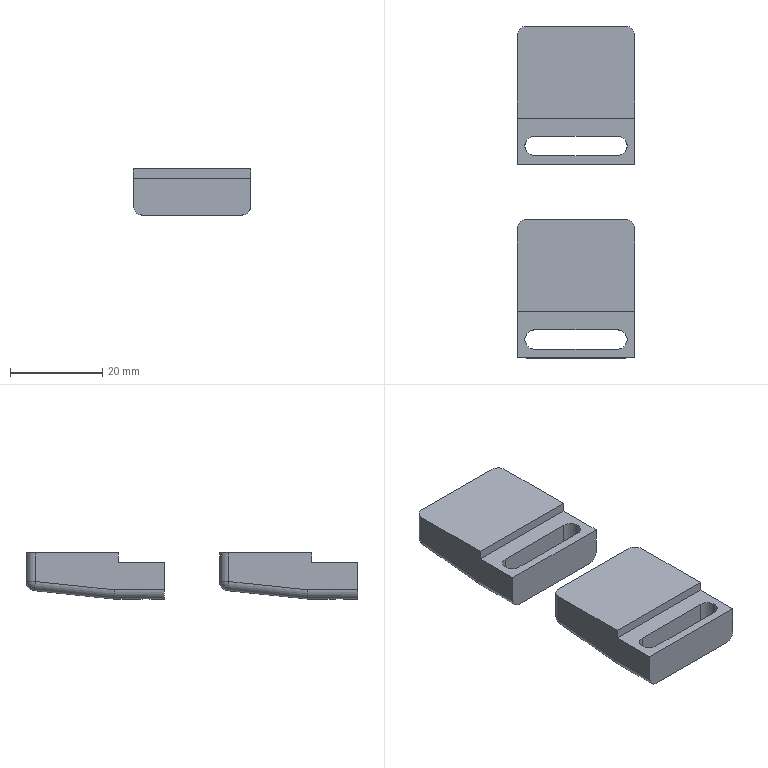NC program | NX | posted with a generic post | part box 25.5 x 72 x 10 mm
Lines 50360 to 51151 of 60534:
(FIXED_CONTOUR_COPY , TOOL : R2)
N100706 T18 M6
N100708 G54
N100710 G17 G0 G90 X23.999 Y-2.844 B0. C0. S9500 M3
N100712 G43 Z30. H18
N100714 Z2.8
N100716 G94 G1 Z-1.939 F1000.
N100718 X23.986 Y-2.857 Z-1.906 F2500.
N100720 X23.923 Y-2.92 Z-1.669
N100722 X23.857 Y-2.919 Z-1.674
N100724 X23.919 Y-2.857 Z-1.906
N100726 X24. Y-2.775 Z-2.113
N100728 Y-2.745 Z-2.188
N100730 Y-2.712 Z-2.252
N100732 Z-2.267
N100734 X23.915 Y-2.797 Z-2.061
N100736 X23.855 Y-2.857 Z-1.907
N100738 X23.794 Y-2.918 Z-1.678
N100740 X23.75 Y-2.917 Z-1.68
N100742 X23.811 Y-2.857 Z-1.907
N100744 X23.864 Y-2.803 Z-2.046
N100746 X23.974 Y-2.693 Z-2.311
N100748 X24. Y-2.668 Z-2.357
N100750 Z-2.339
N100752 Y-2.579 Z-2.512
N100754 X23.999 Z-2.515
N100756 X23.884 Y-2.693 Z-2.311
N100758 X23.837 Y-2.74 Z-2.199
N100760 X23.762 Y-2.815 Z-2.016
N100762 X23.724 Y-2.854 Z-1.915
N100764 X23.662 Y-2.916 Z-1.686
N100766 X23.596 Y-2.915 Z-1.69
N100768 X23.639 Y-2.872 Z-1.85
N100770 X23.664 Y-2.847 Z-1.932
N100772 X23.695 Y-2.816 Z-2.013
N100774 X23.795 Y-2.716 Z-2.259
N100776 X23.818 Y-2.693 Z-2.311
N100778 X23.977 Y-2.534 Z-2.594
N100780 X24. Y-2.511 Z-2.627
N100782 Z-2.618
N100784 Y-2.454 Z-2.701
N100786 Z-2.709
N100788 X23.923 Y-2.531 Z-2.599
N100790 X23.761 Y-2.693 Z-2.311
N100792 X23.738 Y-2.716 Z-2.259
N100794 X23.638 Y-2.816 Z-2.014
N100796 X23.613 Y-2.842 Z-1.947
N100798 X23.573 Y-2.881 Z-1.817
N100800 X23.54 Y-2.914 Z-1.694
N100802 X23.438 Y-2.913 Z-1.7
N100804 X23.453 Y-2.898 Z-1.756
N100806 X23.52 Y-2.832 Z-1.973
N100808 X23.635 Y-2.716 Z-2.26
N100810 X23.652 Y-2.699 Z-2.299
N100812 X23.825 Y-2.526 Z-2.609
N100814 X23.907 Y-2.444 Z-2.724
N100816 X24. Y-2.351 Z-2.85
N100818 Z-2.846
N100820 Y-2.288 Z-2.92
N100822 Z-2.927
N100824 X23.96 Y-2.328 Z-2.881
N100826 X23.844 Y-2.444 Z-2.724
N100828 X23.765 Y-2.523 Z-2.614
N100830 X23.642 Y-2.646 Z-2.393
N100832 X23.585 Y-2.703 Z-2.29
N100834 X23.463 Y-2.825 Z-1.989
N100836 X23.376 Y-2.912 Z-1.704
N100838 X23.273 Y-2.91 Z-1.71
N100840 X23.37 Y-2.814 Z-2.019
N100842 X23.474 Y-2.709 Z-2.276
N100844 X23.564 Y-2.619 Z-2.443
N100846 X23.661 Y-2.522 Z-2.615
N100848 X23.742 Y-2.441 Z-2.728
N100850 X23.855 Y-2.328 Z-2.881
N100852 X23.945 Y-2.238 Z-2.986
N100854 X23.998 Y-2.185 Z-3.042
N100856 Y-2.148 Z-3.08
N100858 X24. Y-2.089 Z-3.136
N100860 Z-3.142
N100862 X23.851 Y-2.238 Z-2.986
N100864 X23.761 Y-2.328 Z-2.881
N100866 X23.567 Y-2.522 Z-2.615
N100868 X23.47 Y-2.619 Z-2.443
N100870 X23.374 Y-2.715 Z-2.264
N100872 X23.276 Y-2.813 Z-2.021
N100874 X23.18 Y-2.909 Z-1.716
N100876 X23.078 Y-2.907 Z-1.723
N100878 X23.173 Y-2.812 Z-2.023
N100880 X23.269 Y-2.716 Z-2.262
N100882 X23.366 Y-2.619 Z-2.443
N100884 X23.463 Y-2.522 Z-2.615
N100886 X23.657 Y-2.328 Z-2.881
N100888 X23.748 Y-2.237 Z-2.987
N100890 X23.947 Y-2.038 Z-3.196
N100892 X24. Y-1.985 Z-3.239
N100894 X23.998 Y-1.883 Z-3.323
N100896 X23.843 Y-2.038 Z-3.196
N100898 X23.666 Y-2.216 Z-3.01
N100900 X23.553 Y-2.328 Z-2.881
N100902 X23.359 Y-2.522 Z-2.615
N100904 X23.232 Y-2.649 Z-2.388
N100906 X23.165 Y-2.716 Z-2.262
N100908 X23.07 Y-2.812 Z-2.025
N100910 X22.975 Y-2.906 Z-1.729
N100912 X22.872 Y-2.904 Z-1.736
N100914 X22.966 Y-2.811 Z-2.026
N100916 X23.06 Y-2.716 Z-2.263
N100918 X23.157 Y-2.619 Z-2.443
N100920 X23.254 Y-2.522 Z-2.615
N100922 X23.449 Y-2.328 Z-2.881
N100924 X23.583 Y-2.194 Z-3.032
N100926 X23.741 Y-2.036 Z-3.198
N100928 X23.978 Y-1.798 Z-3.392
N100930 X23.998 Y-1.778 Z-3.407
N100932 X24. Y-1.757 Z-3.422
N100934 Y-1.684 Z-3.468
N100936 Z-3.474
N100938 X23.885 Y-1.798 Z-3.392
N100940 X23.666 Y-2.017 Z-3.213
N100942 X23.611 Y-2.072 Z-3.16
N100944 X23.509 Y-2.175 Z-3.053
N100946 X23.355 Y-2.328 Z-2.88
N100948 X23.161 Y-2.522 Z-2.616
N100950 X23.064 Y-2.619 Z-2.443
N100952 X22.967 Y-2.716 Z-2.264
N100954 X22.873 Y-2.81 Z-2.028
N100956 X22.781 Y-2.903 Z-1.742
N100958 X22.697 Y-2.902 Z-1.747
N100960 X22.789 Y-2.81 Z-2.03
N100962 X22.883 Y-2.716 Z-2.264
N100964 X22.98 Y-2.619 Z-2.443
N100966 X23.077 Y-2.522 Z-2.616
N100968 X23.271 Y-2.328 Z-2.881
N100970 X23.442 Y-2.157 Z-3.071
N100972 X23.5 Y-2.099 Z-3.132
N100974 X23.598 Y-2. Z-3.227
N100976 X23.8 Y-1.798 Z-3.392
N100978 X23.878 Y-1.721 Z-3.45
N100980 X24. Y-1.599 Z-3.527
N100982 Z-3.52
N100984 Y-1.514 Z-3.573
N100986 Z-3.58
N100988 X23.772 Y-1.742 Z-3.437
N100990 X23.53 Y-1.984 Z-3.241
N100992 X23.375 Y-2.139 Z-3.09
N100994 X23.186 Y-2.328 Z-2.881
N100996 X22.992 Y-2.522 Z-2.616
N100998 X22.875 Y-2.639 Z-2.406
N101000 X22.798 Y-2.716 Z-2.264
N101002 X22.705 Y-2.809 Z-2.031
N101004 X22.614 Y-2.9 Z-1.752
N101006 X22.511 Y-2.899 Z-1.759
N101008 X22.601 Y-2.808 Z-2.033
N101010 X22.694 Y-2.716 Z-2.265
N101012 X22.791 Y-2.619 Z-2.443
N101014 X22.888 Y-2.522 Z-2.616
N101016 X23.082 Y-2.328 Z-2.881
N101018 X23.276 Y-2.134 Z-3.095
N101020 X23.447 Y-1.963 Z-3.258
N101022 X23.664 Y-1.746 Z-3.435
N101024 X23.971 Y-1.439 Z-3.627
N101026 X24. Y-1.41 Z-3.641
N101028 Z-3.638
N101030 X23.998 Y-1.382 Z-3.655
N101032 X24. Y-1.334 Z-3.676
N101034 Y-1.306 Z-3.688
N101036 Z-3.691
N101038 X23.867 Y-1.439 Z-3.627
N101040 X23.56 Y-1.746 Z-3.435
N101042 X23.354 Y-1.951 Z-3.266
N101044 X23.171 Y-2.134 Z-3.095
N101046 X22.977 Y-2.328 Z-2.881
N101048 X22.783 Y-2.522 Z-2.616
N101050 X22.686 Y-2.619 Z-2.443
N101052 X22.589 Y-2.716 Z-2.265
N101054 X22.498 Y-2.808 Z-2.035
N101056 X22.408 Y-2.897 Z-1.765
N101058 X22.319 Y-2.896 Z-1.771
N101060 X22.408 Y-2.807 Z-2.036
N101062 X22.499 Y-2.716 Z-2.265
N101064 X22.596 Y-2.619 Z-2.443
N101066 X22.693 Y-2.522 Z-2.616
N101068 X22.887 Y-2.328 Z-2.881
N101070 X23.081 Y-2.134 Z-3.095
N101072 X23.275 Y-1.94 Z-3.276
N101074 X23.469 Y-1.746 Z-3.435
N101076 X23.776 Y-1.439 Z-3.627
N101078 X24. Y-1.215 Z-3.733
N101080 Z-3.726
N101082 Y-1.124 Z-3.765
N101084 Z-3.774
N101086 X23.696 Y-1.428 Z-3.633
N101088 X23.658 Y-1.465 Z-3.611
N101090 X23.378 Y-1.746 Z-3.435
N101092 X23.184 Y-1.94 Z-3.276
N101094 X22.99 Y-2.134 Z-3.095
N101096 X22.796 Y-2.328 Z-2.881
N101098 X22.602 Y-2.522 Z-2.616
N101100 X22.505 Y-2.619 Z-2.443
N101102 X22.408 Y-2.716 Z-2.266
N101104 X22.318 Y-2.806 Z-2.038
N101106 X22.229 Y-2.895 Z-1.776
N101108 X22.127 Y-2.893 Z-1.783
N101110 X22.214 Y-2.805 Z-2.04
N101112 X22.304 Y-2.716 Z-2.266
N101114 X22.432 Y-2.588 Z-2.499
N101116 X22.498 Y-2.522 Z-2.616
N101118 X22.692 Y-2.328 Z-2.881
N101120 X22.886 Y-2.134 Z-3.095
N101122 X23.08 Y-1.94 Z-3.276
N101124 X23.274 Y-1.746 Z-3.435
N101126 X23.513 Y-1.507 Z-3.585
N101128 X23.61 Y-1.41 Z-3.641
N101130 X23.856 Y-1.164 Z-3.757
N101132 X23.946 Y-1.074 Z-3.796
N101134 X24. Y-1.02 Z-3.813
N101136 Z-3.81
N101138 X23.998 Y-0.987 Z-3.824
N101140 X24. Y-0.961 Z-3.832
N101142 Y-0.916 Z-3.843
N101144 Z-3.846
N101146 X23.842 Y-1.074 Z-3.796
N101148 X23.751 Y-1.164 Z-3.756
N101150 X23.524 Y-1.392 Z-3.65
N101152 X23.368 Y-1.548 Z-3.559
N101154 X23.17 Y-1.746 Z-3.435
N101156 X22.976 Y-1.94 Z-3.276
N101158 X22.782 Y-2.134 Z-3.095
N101160 X22.588 Y-2.328 Z-2.881
N101162 X22.394 Y-2.522 Z-2.616
N101164 X22.2 Y-2.716 Z-2.266
N101166 X22.111 Y-2.805 Z-2.042
N101168 X22.024 Y-2.892 Z-1.789
N101170 X21.93 Y-2.89 Z-1.795
N101172 X22.017 Y-2.804 Z-2.044
N101174 X22.104 Y-2.716 Z-2.266
N101176 X22.299 Y-2.522 Z-2.617
N101178 X22.493 Y-2.328 Z-2.881
N101180 X22.687 Y-2.134 Z-3.095
N101182 X22.881 Y-1.94 Z-3.276
N101184 X23.075 Y-1.746 Z-3.435
N101186 X23.269 Y-1.552 Z-3.556
N101188 X23.445 Y-1.376 Z-3.658
N101190 X23.657 Y-1.164 Z-3.757
N101192 X23.688 Y-1.133 Z-3.768
N101194 X23.748 Y-1.073 Z-3.796
N101196 X24. Y-0.821 Z-3.877
N101198 Z-3.869
N101200 Y-0.725 Z-3.895
N101202 Z-3.904
N101204 X23.949 Y-0.776 Z-3.892
N101206 X23.672 Y-1.053 Z-3.803
N101208 X23.623 Y-1.101 Z-3.78
N101210 X23.561 Y-1.164 Z-3.757
N101212 X23.354 Y-1.37 Z-3.659
N101214 X23.173 Y-1.552 Z-3.556
N101216 X22.979 Y-1.746 Z-3.435
N101218 X22.784 Y-1.94 Z-3.276
N101220 X22.59 Y-2.134 Z-3.095
N101222 X22.396 Y-2.328 Z-2.881
N101224 X22.202 Y-2.522 Z-2.617
N101226 X22.008 Y-2.716 Z-2.266
N101228 X21.921 Y-2.803 Z-2.045
N101230 X21.835 Y-2.889 Z-1.801
N101232 X21.733 Y-2.888 Z-1.808
N101234 X21.818 Y-2.802 Z-2.047
N101236 X21.905 Y-2.716 Z-2.266
N101238 X22.099 Y-2.522 Z-2.617
N101240 X22.293 Y-2.328 Z-2.881
N101242 X22.487 Y-2.134 Z-3.095
N101244 X22.681 Y-1.94 Z-3.276
N101246 X22.875 Y-1.746 Z-3.435
N101248 X23.069 Y-1.552 Z-3.556
N101250 X23.263 Y-1.358 Z-3.666
N101252 X23.457 Y-1.164 Z-3.757
N101254 X23.554 Y-1.067 Z-3.793
N101256 X23.59 Y-1.031 Z-3.809
N101258 X23.845 Y-0.776 Z-3.892
N101260 X23.935 Y-0.686 Z-3.914
N101262 X24. Y-0.621 Z-3.926
N101264 Z-3.923
N101266 X23.998 Y-0.592 Z-3.931
N101268 X24. Y-0.557 Z-3.938
N101270 Y-0.518 Z-3.943
N101272 Z-3.945
N101274 X23.832 Y-0.686 Z-3.914
N101276 X23.742 Y-0.776 Z-3.892
N101278 X23.507 Y-1.01 Z-3.816
N101280 X23.484 Y-1.033 Z-3.806
N101282 X23.353 Y-1.165 Z-3.756
N101284 X23.159 Y-1.358 Z-3.666
N101286 X22.965 Y-1.552 Z-3.556
N101288 X22.771 Y-1.746 Z-3.435
N101290 X22.577 Y-1.94 Z-3.276
N101292 X22.383 Y-2.134 Z-3.095
N101294 X22.189 Y-2.328 Z-2.881
N101296 X21.995 Y-2.522 Z-2.617
N101298 X21.801 Y-2.716 Z-2.266
N101300 X21.716 Y-2.802 Z-2.049
N101302 X21.631 Y-2.886 Z-1.814
N101304 X21.534 Y-2.885 Z-1.82
N101306 X21.618 Y-2.801 Z-2.051
N101308 X21.703 Y-2.716 Z-2.266
N101310 X21.897 Y-2.522 Z-2.618
N101312 X22.091 Y-2.328 Z-2.881
N101314 X22.285 Y-2.134 Z-3.095
N101316 X22.479 Y-1.94 Z-3.276
N101318 X22.673 Y-1.746 Z-3.435
N101320 X22.867 Y-1.552 Z-3.556
N101322 X23.061 Y-1.358 Z-3.666
N101324 X23.255 Y-1.164 Z-3.757
N101326 X23.43 Y-0.989 Z-3.823
N101328 X23.643 Y-0.776 Z-3.892
N101330 X23.737 Y-0.682 Z-3.914
N101332 X24. Y-0.419 Z-3.964
N101334 Z-3.958
N101336 Y-0.32 Z-3.973
N101338 Z-3.978
N101340 X23.933 Y-0.388 Z-3.97
N101342 X23.659 Y-0.661 Z-3.918
N101344 X23.544 Y-0.776 Z-3.892
N101346 X23.35 Y-0.97 Z-3.829
N101348 X23.156 Y-1.164 Z-3.757
N101350 X22.962 Y-1.358 Z-3.666
N101352 X22.768 Y-1.552 Z-3.556
N101354 X22.574 Y-1.746 Z-3.435
N101356 X22.38 Y-1.94 Z-3.276
N101358 X22.186 Y-2.134 Z-3.095
N101360 X21.992 Y-2.328 Z-2.881
N101362 X21.798 Y-2.522 Z-2.618
N101364 X21.604 Y-2.716 Z-2.266
N101366 X21.52 Y-2.8 Z-2.053
N101368 X21.437 Y-2.883 Z-1.827
N101370 X21.335 Y-2.882 Z-1.833
N101372 X21.417 Y-2.799 Z-2.055
N101374 X21.5 Y-2.716 Z-2.266
N101376 X21.694 Y-2.522 Z-2.618
N101378 X21.888 Y-2.328 Z-2.881
N101380 X22.082 Y-2.134 Z-3.095
N101382 X22.277 Y-1.94 Z-3.276
N101384 X22.471 Y-1.746 Z-3.435
N101386 X22.665 Y-1.552 Z-3.556
N101388 X22.859 Y-1.358 Z-3.666
N101390 X23.053 Y-1.164 Z-3.757
N101392 X23.247 Y-0.97 Z-3.829
N101394 X23.441 Y-0.776 Z-3.892
N101396 X23.577 Y-0.64 Z-3.922
N101398 X23.829 Y-0.388 Z-3.97
N101400 X24. Y-0.217 Z-3.99
N101402 Y-0.168 Z-3.992
N101404 Y-0.113
N101406 Z-3.995
N101408 X23.877 Y-0.235 Z-3.989
N101410 X23.725 Y-0.388 Z-3.97
N101412 X23.494 Y-0.618 Z-3.926
N101414 X23.337 Y-0.776 Z-3.892
N101416 X23.143 Y-0.97 Z-3.829
N101418 X22.949 Y-1.164 Z-3.757
N101420 X22.755 Y-1.358 Z-3.666
N101422 X22.56 Y-1.552 Z-3.556
N101424 X22.367 Y-1.746 Z-3.435
N101426 X22.173 Y-1.94 Z-3.276
N101428 X21.978 Y-2.134 Z-3.095
N101430 X21.784 Y-2.328 Z-2.881
N101432 X21.59 Y-2.522 Z-2.618
N101434 X21.396 Y-2.716 Z-2.266
N101436 X21.314 Y-2.799 Z-2.058
N101438 X21.233 Y-2.88 Z-1.839
N101440 X21.135 Y-2.878 Z-1.846
N101442 X21.215 Y-2.798 Z-2.061
N101444 X21.296 Y-2.716 Z-2.266
N101446 X21.49 Y-2.522 Z-2.618
N101448 X21.684 Y-2.328 Z-2.881
N101450 X21.879 Y-2.134 Z-3.095
N101452 X22.073 Y-1.94 Z-3.276
N101454 X22.267 Y-1.746 Z-3.435
N101456 X22.461 Y-1.552 Z-3.556
N101458 X22.655 Y-1.358 Z-3.666
N101460 X22.849 Y-1.164 Z-3.757
N101462 X23.043 Y-0.97 Z-3.829
N101464 X23.237 Y-0.776 Z-3.892
N101466 X23.415 Y-0.598 Z-3.93
N101468 X23.625 Y-0.388 Z-3.97
N101470 X23.809 Y-0.203 Z-3.992
N101472 X24. Y-0.013 Z-3.999
N101474 Z-3.992
N101476 Y0.087
N101478 Z-3.996
N101480 X23.913 Y0.001 Z-3.999
N101482 X23.719 Y-0.193 Z-3.993
N101484 X23.525 Y-0.388 Z-3.97
N101486 X23.331 Y-0.582 Z-3.933
N101488 X23.137 Y-0.776 Z-3.892
N101490 X22.943 Y-0.97 Z-3.829
N101492 X22.749 Y-1.164 Z-3.757
N101494 X22.555 Y-1.358 Z-3.666
N101496 X22.361 Y-1.552 Z-3.556
N101498 X22.167 Y-1.746 Z-3.435
N101500 X21.973 Y-1.94 Z-3.276
N101502 X21.779 Y-2.134 Z-3.095
N101504 X21.584 Y-2.328 Z-2.881
N101506 X21.39 Y-2.522 Z-2.619
N101508 X21.196 Y-2.716 Z-2.266
N101510 X21.116 Y-2.797 Z-2.064
N101512 X21.037 Y-2.876 Z-1.852
N101514 X20.934 Y-2.874 Z-1.858
N101516 X21.022 Y-2.785 Z-2.094
N101518 X21.091 Y-2.716 Z-2.266
N101520 X21.285 Y-2.522 Z-2.619
N101522 X21.479 Y-2.328 Z-2.881
N101524 X21.673 Y-2.134 Z-3.095
N101526 X21.867 Y-1.94 Z-3.276
N101528 X22.061 Y-1.746 Z-3.435
N101530 X22.256 Y-1.552 Z-3.556
N101532 X22.45 Y-1.358 Z-3.666
N101534 X22.644 Y-1.164 Z-3.757
N101536 X22.838 Y-0.97 Z-3.829
N101538 X23.032 Y-0.776 Z-3.892
N101540 X23.226 Y-0.582 Z-3.933
N101542 X23.42 Y-0.388 Z-3.97
N101544 X23.614 Y-0.193 Z-3.993
N101546 X23.808 Y0.001 Z-3.999
N101548 X23.998 Y0.191 Z-3.991
N101550 X24. Y0.218 Z-3.989
N101552 Y0.298 Z-3.977
N101554 Z-3.981
N101556 X23.926 Y0.224 Z-3.99
N101558 X23.796 Y0.094 Z-3.996
N101560 X23.702 Y0.001 Z-3.999
N101562 X23.494 Y-0.208 Z-3.991
N101564 X23.314 Y-0.388 Z-3.97
N101566 X23.12 Y-0.582 Z-3.933
N101568 X22.926 Y-0.776 Z-3.892
N101570 X22.732 Y-0.97 Z-3.829
N101572 X22.538 Y-1.164 Z-3.757
N101574 X22.344 Y-1.358 Z-3.666
N101576 X22.15 Y-1.552 Z-3.556
N101578 X21.956 Y-1.746 Z-3.435
N101580 X21.762 Y-1.94 Z-3.276
N101582 X21.568 Y-2.134 Z-3.095
N101584 X21.374 Y-2.328 Z-2.881
N101586 X21.18 Y-2.522 Z-2.619
N101588 X20.986 Y-2.716 Z-2.266
N101590 X20.892 Y-2.809 Z-2.031
N101592 X20.83 Y-2.872 Z-1.865
N101594 X20.727 Y-2.87 Z-1.871
N101596 X20.803 Y-2.794 Z-2.074
N101598 X20.88 Y-2.716 Z-2.266
N101600 X21.074 Y-2.522 Z-2.619
N101602 X21.268 Y-2.328 Z-2.881
N101604 X21.462 Y-2.134 Z-3.095
N101606 X21.656 Y-1.94 Z-3.276
N101608 X21.85 Y-1.746 Z-3.435
N101610 X22.044 Y-1.552 Z-3.556
N101612 X22.238 Y-1.358 Z-3.666
N101614 X22.433 Y-1.164 Z-3.757
N101616 X22.627 Y-0.97 Z-3.829
N101618 X22.821 Y-0.776 Z-3.892
N101620 X23.015 Y-0.582 Z-3.933
N101622 X23.209 Y-0.388 Z-3.97
N101624 X23.403 Y-0.193 Z-3.993
N101626 X23.597 Y0.001 Z-3.999
N101628 X23.799 Y0.203 Z-3.992
N101630 X24. Y0.403 Z-3.967
N101632 Z-3.96
N101634 Y0.509 Z-3.944
N101636 Z-3.947
N101638 X23.879 Y0.389 Z-3.97
N101640 X23.685 Y0.195 Z-3.992
N101642 X23.491 Y0.001 Z-3.999
N101644 X23.297 Y-0.193 Z-3.993
N101646 X23.103 Y-0.388 Z-3.97
N101648 X22.909 Y-0.582 Z-3.933
N101650 X22.715 Y-0.776 Z-3.892
N101652 X22.521 Y-0.97 Z-3.829
N101654 X22.327 Y-1.164 Z-3.757
N101656 X22.133 Y-1.358 Z-3.666
N101658 X21.939 Y-1.552 Z-3.556
N101660 X21.745 Y-1.746 Z-3.435
N101662 X21.551 Y-1.94 Z-3.276
N101664 X21.357 Y-2.134 Z-3.095
N101666 X21.163 Y-2.328 Z-2.881
N101668 X20.969 Y-2.522 Z-2.619
N101670 X20.774 Y-2.716 Z-2.266
N101672 X20.698 Y-2.793 Z-2.078
N101674 X20.623 Y-2.867 Z-1.878
N101676 X20.52 Y-2.865 Z-1.884
N101678 X20.594 Y-2.791 Z-2.081
N101680 X20.669 Y-2.716 Z-2.266
N101682 X20.863 Y-2.522 Z-2.619
N101684 X21.057 Y-2.328 Z-2.881
N101686 X21.251 Y-2.134 Z-3.095
N101688 X21.445 Y-1.94 Z-3.276
N101690 X21.639 Y-1.746 Z-3.435
N101692 X21.833 Y-1.552 Z-3.556
N101694 X22.027 Y-1.358 Z-3.666
N101696 X22.221 Y-1.164 Z-3.757
N101698 X22.415 Y-0.97 Z-3.829
N101700 X22.609 Y-0.776 Z-3.892
N101702 X22.803 Y-0.582 Z-3.933
N101704 X22.997 Y-0.388 Z-3.97
N101706 X23.192 Y-0.193 Z-3.993
N101708 X23.386 Y0.001 Z-3.999
N101710 X23.58 Y0.195 Z-3.992
N101712 X23.774 Y0.389 Z-3.97
N101714 X24. Y0.615 Z-3.927
N101716 Z-3.925
N101718 Y0.715 Z-3.898
N101720 Z-3.907
N101722 X23.972 Y0.687 Z-3.913
N101724 X23.674 Y0.389 Z-3.97
N101726 X23.48 Y0.195 Z-3.992
N101728 X23.286 Y0.001 Z-3.999
N101730 X23.092 Y-0.193 Z-3.993
N101732 X22.897 Y-0.388 Z-3.97
N101734 X22.703 Y-0.582 Z-3.933
N101736 X22.509 Y-0.776 Z-3.892
N101738 X22.315 Y-0.97 Z-3.829
N101740 X22.121 Y-1.164 Z-3.757
N101742 X21.927 Y-1.358 Z-3.666
N101744 X21.733 Y-1.552 Z-3.556
N101746 X21.539 Y-1.746 Z-3.435
N101748 X21.345 Y-1.94 Z-3.276
N101750 X21.151 Y-2.134 Z-3.095
N101752 X20.957 Y-2.328 Z-2.881
N101754 X20.763 Y-2.522 Z-2.619
N101756 X20.569 Y-2.716 Z-2.266
N101758 X20.494 Y-2.79 Z-2.084
N101760 X20.422 Y-2.863 Z-1.891
N101762 X20.323 Y-2.862 Z-1.897
N101764 X20.395 Y-2.79 Z-2.088
N101766 X20.469 Y-2.716 Z-2.267
N101768 X20.663 Y-2.522 Z-2.619
N101770 X20.857 Y-2.328 Z-2.881
N101772 X21.051 Y-2.134 Z-3.095
N101774 X21.245 Y-1.94 Z-3.276
N101776 X21.439 Y-1.746 Z-3.435
N101778 X21.633 Y-1.552 Z-3.556
N101780 X21.827 Y-1.358 Z-3.666
N101782 X22.021 Y-1.164 Z-3.757
N101784 X22.215 Y-0.97 Z-3.829
N101786 X22.409 Y-0.776 Z-3.892
N101788 X22.603 Y-0.582 Z-3.933
N101790 X22.797 Y-0.388 Z-3.97
N101792 X22.992 Y-0.193 Z-3.993
N101794 X23.186 Y0.001 Z-3.999
N101796 X23.38 Y0.195 Z-3.992
N101798 X23.574 Y0.389 Z-3.97
N101800 X23.872 Y0.687 Z-3.913
N101802 X23.962 Y0.777 Z-3.891
N101804 X24. Y0.815 Z-3.879
N101806 Z-3.871
N101808 Y0.915 Z-3.843
N101810 Z-3.847
N101812 X23.862 Y0.777 Z-3.891
N101814 X23.751 Y0.666 Z-3.917
N101816 X23.474 Y0.389 Z-3.97
N101818 X23.28 Y0.195 Z-3.992
N101820 X23.086 Y0.001 Z-3.999
N101822 X22.892 Y-0.193 Z-3.993
N101824 X22.697 Y-0.388 Z-3.97
N101826 X22.503 Y-0.582 Z-3.933
N101828 X22.309 Y-0.776 Z-3.892
N101830 X22.115 Y-0.97 Z-3.829
N101832 X21.921 Y-1.164 Z-3.757
N101834 X21.727 Y-1.358 Z-3.666
N101836 X21.533 Y-1.552 Z-3.556
N101838 X21.339 Y-1.746 Z-3.435
N101840 X21.145 Y-1.94 Z-3.276
N101842 X20.951 Y-2.134 Z-3.095
N101844 X20.757 Y-2.328 Z-2.881
N101846 X20.563 Y-2.522 Z-2.619
N101848 X20.369 Y-2.716 Z-2.267
N101850 X20.296 Y-2.789 Z-2.091
N101852 X20.226 Y-2.859 Z-1.903
N101854 X20.122 Y-2.858 Z-1.909
N101856 X20.192 Y-2.787 Z-2.094
N101858 X20.263 Y-2.716 Z-2.267
N101860 X20.457 Y-2.522 Z-2.619
N101862 X20.651 Y-2.328 Z-2.881
N101864 X20.845 Y-2.134 Z-3.095
N101866 X21.039 Y-1.94 Z-3.276
N101868 X21.233 Y-1.746 Z-3.435
N101870 X21.427 Y-1.552 Z-3.556
N101872 X21.621 Y-1.358 Z-3.666
N101874 X21.815 Y-1.164 Z-3.757
N101876 X22.009 Y-0.97 Z-3.829
N101878 X22.203 Y-0.776 Z-3.892
N101880 X22.398 Y-0.582 Z-3.933
N101882 X22.592 Y-0.388 Z-3.97
N101884 X22.786 Y-0.193 Z-3.993
N101886 X22.98 Y0.001 Z-3.999
N101888 X23.174 Y0.195 Z-3.992
N101890 X23.368 Y0.389 Z-3.97
N101892 X23.682 Y0.703 Z-3.91
N101894 X23.755 Y0.776 Z-3.892
N101896 X24. Y1.021 Z-3.813
N101898 Z-3.809
N101900 Y1.12 Z-3.767
N101902 Z-3.776
N101904 X23.954 Y1.075 Z-3.795
N101906 X23.656 Y0.777 Z-3.891
N101908 X23.6 Y0.721 Z-3.905
N101910 X23.268 Y0.389 Z-3.97
N101912 X23.074 Y0.195 Z-3.992
N101914 X22.88 Y0.001 Z-3.999
N101916 X22.686 Y-0.193 Z-3.993
N101918 X22.492 Y-0.388 Z-3.97
N101920 X22.298 Y-0.582 Z-3.933
N101922 X22.104 Y-0.776 Z-3.892
N101924 X21.909 Y-0.97 Z-3.829
N101926 X21.715 Y-1.164 Z-3.757
N101928 X21.521 Y-1.358 Z-3.666
N101930 X21.327 Y-1.552 Z-3.556
N101932 X21.133 Y-1.746 Z-3.435
N101934 X20.939 Y-1.94 Z-3.276
N101936 X20.745 Y-2.134 Z-3.095
N101938 X20.551 Y-2.328 Z-2.881
N101940 X20.357 Y-2.522 Z-2.619
N101942 X20.163 Y-2.716 Z-2.267
N101944 X20.093 Y-2.786 Z-2.098
N101946 X20.024 Y-2.856 Z-1.916
N101948 X19.926 Y-2.854 Z-1.922
N101950 X19.994 Y-2.785 Z-2.101
N101952 X20.063 Y-2.716 Z-2.267
N101954 X20.257 Y-2.522 Z-2.619
N101956 X20.451 Y-2.328 Z-2.881
N101958 X20.645 Y-2.134 Z-3.095
N101960 X20.839 Y-1.94 Z-3.276
N101962 X21.033 Y-1.746 Z-3.435
N101964 X21.227 Y-1.552 Z-3.556
N101966 X21.421 Y-1.358 Z-3.666
N101968 X21.615 Y-1.164 Z-3.757
N101970 X21.81 Y-0.97 Z-3.829
N101972 X22.004 Y-0.776 Z-3.892
N101974 X22.198 Y-0.582 Z-3.933
N101976 X22.392 Y-0.388 Z-3.97
N101978 X22.586 Y-0.193 Z-3.993
N101980 X22.78 Y0.001 Z-3.999
N101982 X22.974 Y0.195 Z-3.992
N101984 X23.168 Y0.389 Z-3.97
N101986 X23.359 Y0.58 Z-3.934
N101988 X23.556 Y0.777 Z-3.891
N101990 X23.854 Y1.075 Z-3.795
N101992 X24. Y1.22 Z-3.73
N101994 Z-3.724
N101996 Y1.32 Z-3.682
N101998 Z-3.683
N102000 X23.845 Y1.165 Z-3.756
N102002 X23.754 Y1.074 Z-3.796
N102004 X23.456 Y0.777 Z-3.891
N102006 X23.262 Y0.583 Z-3.933
N102008 X23.068 Y0.389 Z-3.97
N102010 X22.874 Y0.195 Z-3.992
N102012 X22.68 Y0.001 Z-3.999
N102014 X22.486 Y-0.193 Z-3.993
N102016 X22.292 Y-0.388 Z-3.97
N102018 X22.098 Y-0.582 Z-3.933
N102020 X21.904 Y-0.776 Z-3.892
N102022 X21.71 Y-0.97 Z-3.829
N102024 X21.516 Y-1.164 Z-3.757
N102026 X21.322 Y-1.358 Z-3.666
N102028 X21.128 Y-1.552 Z-3.556
N102030 X20.934 Y-1.746 Z-3.435
N102032 X20.74 Y-1.94 Z-3.276
N102034 X20.546 Y-2.134 Z-3.095
N102036 X20.351 Y-2.328 Z-2.881
N102038 X20.157 Y-2.522 Z-2.619
N102040 X19.963 Y-2.716 Z-2.267
N102042 X19.895 Y-2.784 Z-2.104
N102044 X19.828 Y-2.852 Z-1.928
N102046 X19.731 Y-2.85 Z-1.934
N102048 X19.797 Y-2.784 Z-2.107
N102050 X19.864 Y-2.716 Z-2.267
N102052 X20.058 Y-2.522 Z-2.619
N102054 X20.252 Y-2.328 Z-2.881
N102056 X20.446 Y-2.134 Z-3.095
N102058 X20.641 Y-1.94 Z-3.276
N102060 X20.835 Y-1.746 Z-3.435
N102062 X21.029 Y-1.552 Z-3.556
N102064 X21.223 Y-1.358 Z-3.666
N102066 X21.417 Y-1.164 Z-3.757
N102068 X21.611 Y-0.97 Z-3.829
N102070 X21.805 Y-0.776 Z-3.892
N102072 X21.999 Y-0.582 Z-3.933
N102074 X22.193 Y-0.388 Z-3.97
N102076 X22.387 Y-0.193 Z-3.993
N102078 X22.581 Y0.001 Z-3.999
N102080 X22.775 Y0.195 Z-3.992
N102082 X22.969 Y0.389 Z-3.97
N102084 X23.163 Y0.583 Z-3.933
N102086 X23.357 Y0.776 Z-3.891
N102088 X23.621 Y1.041 Z-3.806
N102090 X23.673 Y1.093 Z-3.788
N102092 X23.857 Y1.276 Z-3.704
N102094 X24. Y1.419 Z-3.637
N102096 Z-3.632
N102098 Y1.525 Z-3.566
N102100 Z-3.573
N102102 X23.914 Y1.439 Z-3.627
N102104 X23.64 Y1.165 Z-3.756
N102106 X23.587 Y1.112 Z-3.779
N102108 X23.478 Y1.003 Z-3.818
N102110 X23.252 Y0.777 Z-3.891
N102112 X23.058 Y0.583 Z-3.933
N102114 X22.863 Y0.389 Z-3.97
N102116 X22.669 Y0.195 Z-3.992
N102118 X22.475 Y0.001 Z-3.999
N102120 X22.281 Y-0.193 Z-3.993
N102122 X22.087 Y-0.388 Z-3.97
N102124 X21.893 Y-0.582 Z-3.933
N102126 X21.699 Y-0.776 Z-3.892
N102128 X21.505 Y-0.97 Z-3.829
N102130 X21.311 Y-1.164 Z-3.757
N102132 X21.117 Y-1.358 Z-3.666
N102134 X20.923 Y-1.552 Z-3.556
N102136 X20.729 Y-1.746 Z-3.435
N102138 X20.535 Y-1.94 Z-3.276
N102140 X20.341 Y-2.134 Z-3.095
N102142 X20.147 Y-2.328 Z-2.881
N102144 X19.953 Y-2.522 Z-2.619
N102146 X19.759 Y-2.716 Z-2.267
N102148 X19.676 Y-2.799 Z-2.068
N102150 X19.627 Y-2.847 Z-1.941
N102152 X19.524 Y-2.845 Z-1.947
N102154 X19.614 Y-2.755 Z-2.175
N102156 X19.653 Y-2.716 Z-2.267
N102158 X19.847 Y-2.522 Z-2.619
N102160 X20.041 Y-2.328 Z-2.881
N102162 X20.235 Y-2.134 Z-3.095
N102164 X20.429 Y-1.94 Z-3.276
N102166 X20.623 Y-1.746 Z-3.435
N102168 X20.817 Y-1.552 Z-3.556
N102170 X21.011 Y-1.358 Z-3.666
N102172 X21.205 Y-1.164 Z-3.757
N102174 X21.399 Y-0.97 Z-3.829
N102176 X21.593 Y-0.776 Z-3.892
N102178 X21.787 Y-0.582 Z-3.933
N102180 X21.981 Y-0.388 Z-3.97
N102182 X22.175 Y-0.193 Z-3.993
N102184 X22.369 Y0.001 Z-3.999
N102186 X22.562 Y0.194 Z-3.993
N102188 X22.758 Y0.389 Z-3.97
N102190 X22.952 Y0.583 Z-3.933
N102192 X23.146 Y0.777 Z-3.891
N102194 X23.354 Y0.985 Z-3.823
N102196 X23.501 Y1.132 Z-3.771
N102198 X23.808 Y1.439 Z-3.627
N102200 X24. Y1.631 Z-3.507
N102202 Z-3.5
N102204 Y1.737 Z-3.435
N102206 Z-3.437
N102208 X23.961 Y1.698 Z-3.465
N102210 X23.751 Y1.488 Z-3.596
N102212 X23.69 Y1.427 Z-3.633
N102214 X23.414 Y1.151 Z-3.762
N102216 X23.234 Y0.971 Z-3.829
N102218 X23.04 Y0.777 Z-3.891
N102220 X22.846 Y0.583 Z-3.933
N102222 X22.652 Y0.389 Z-3.97
N102224 X22.458 Y0.195 Z-3.992
N102226 X22.264 Y0.001 Z-3.999
N102228 X22.07 Y-0.193 Z-3.993
N102230 X21.876 Y-0.388 Z-3.97
N102232 X21.682 Y-0.582 Z-3.933
N102234 X21.487 Y-0.776 Z-3.892
N102236 X21.293 Y-0.97 Z-3.829
N102238 X21.099 Y-1.164 Z-3.757
N102240 X20.905 Y-1.358 Z-3.666
N102242 X20.711 Y-1.552 Z-3.556
N102244 X20.517 Y-1.746 Z-3.435
N102246 X20.323 Y-1.94 Z-3.276
N102248 X20.129 Y-2.134 Z-3.095
N102250 X19.935 Y-2.328 Z-2.881
N102252 X19.741 Y-2.522 Z-2.619
N102254 X19.547 Y-2.716 Z-2.267
N102256 X19.42 Y-2.843 Z-1.953
N102258 X19.316 Y-2.841 Z-1.96
N102260 X19.441 Y-2.716 Z-2.267
N102262 X19.635 Y-2.522 Z-2.619
N102264 X19.829 Y-2.328 Z-2.881
N102266 X20.023 Y-2.134 Z-3.095
N102268 X20.217 Y-1.94 Z-3.276
N102270 X20.411 Y-1.746 Z-3.435
N102272 X20.605 Y-1.552 Z-3.556
N102274 X20.799 Y-1.358 Z-3.666
N102276 X20.993 Y-1.164 Z-3.757
N102278 X21.187 Y-0.97 Z-3.829
N102280 X21.382 Y-0.776 Z-3.892
N102282 X21.576 Y-0.582 Z-3.933